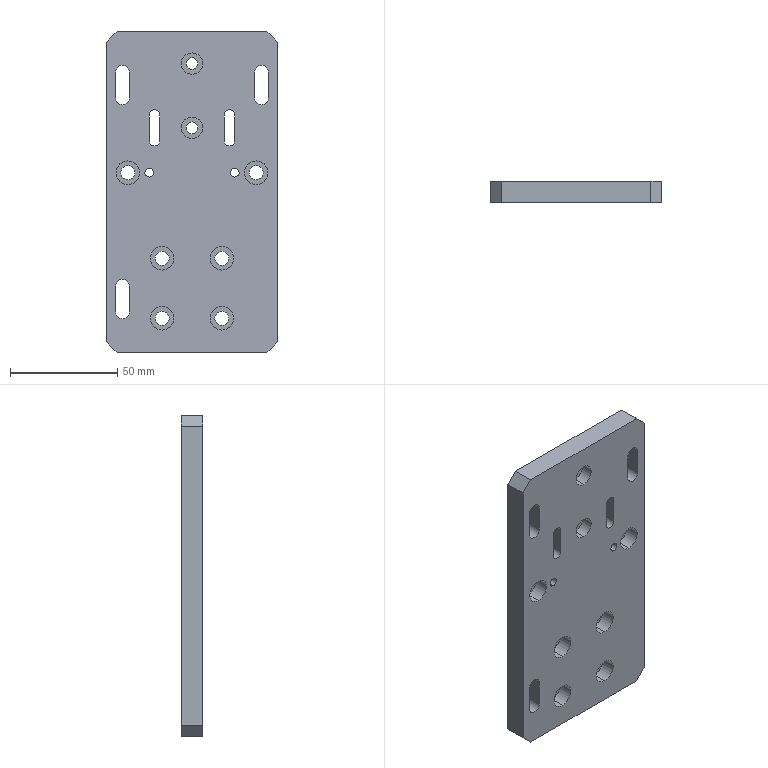Part | STEP file | PN_0037 | 1 solid | 79 faces | box 80 x 10 x 150 mm | volume 108687 mm3 | cylinder 51 | plane 28 | commonest cylinder face diameters 6.6 x12 11 x12 6.5 x9 5 x6 4 x4 5.5 x4